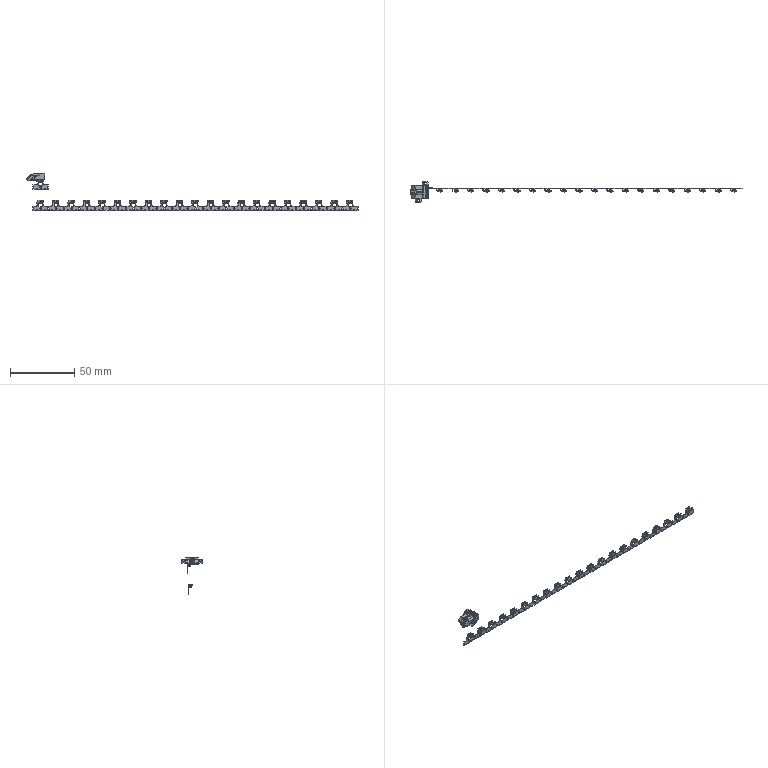Part | NX | 3 solids | 4353 faces | volume 628.895 mm3 | plane 2538 | cylinder 1393 | torus 294 | spline 62 | sphere 48 | cone 18 | commonest cylinder face diameters 0.3 x352 0.2 x230 0.7 x118 1.3 x112 0.5 x111 0.4 x100